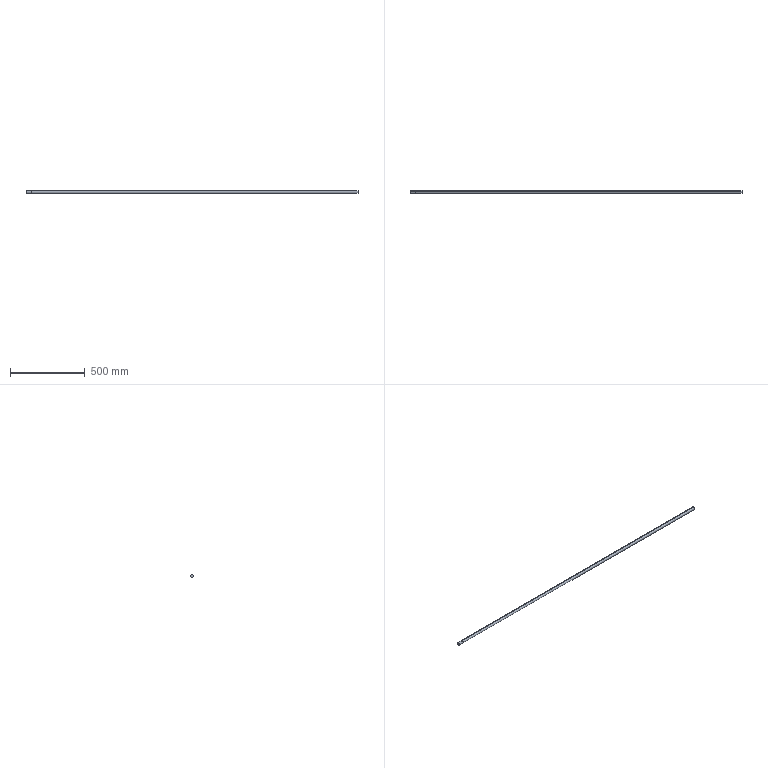Part | STEP file | _MAX100010001N_rod2 | 1 solid | 7 faces | box 2216 x 20 x 20 mm | volume 695277 mm3 | cylinder 4 | plane 3 | commonest cylinder face diameters 19 x2 20 x2
STEP:
#1=CARTESIAN_POINT('',(1723.,0.,-10.));
#2=VERTEX_POINT('',#1);
#3=CARTESIAN_POINT('',(1723.,0.,10.));
#4=VERTEX_POINT('',#3);
#5=CARTESIAN_POINT('',(1723.,0.,0.));
#6=DIRECTION('',(1.,0.,0.));
#7=DIRECTION('',(0.,0.,-1.));
#8=AXIS2_PLACEMENT_3D('',#5,#6,#7);
#9=CIRCLE('',#8,10.);
#10=EDGE_CURVE('',#2,#4,#9,.T.);
#11=ORIENTED_EDGE('',*,*,#10,.F.);
#12=CARTESIAN_POINT('',(-459.,0.,-10.));
#13=VERTEX_POINT('',#12);
#14=CARTESIAN_POINT('',(493.5,0.,-10.));
#15=DIRECTION('',(-1.,0.,0.));
#16=VECTOR('',#15,1000.);
#17=LINE('',#14,#16);
#18=EDGE_CURVE('',#2,#13,#17,.T.);
#19=ORIENTED_EDGE('',*,*,#18,.T.);
#20=CARTESIAN_POINT('',(-459.,0.,10.));
#21=VERTEX_POINT('',#20);
#22=CARTESIAN_POINT('',(-459.,0.,0.));
#23=DIRECTION('',(1.,0.,0.));
#24=DIRECTION('',(0.,0.,1.));
#25=AXIS2_PLACEMENT_3D('',#22,#23,#24);
#26=CIRCLE('',#25,10.);
#27=EDGE_CURVE('',#13,#21,#26,.T.);
#28=ORIENTED_EDGE('',*,*,#27,.T.);
#29=CARTESIAN_POINT('',(493.5,0.,10.));
#30=DIRECTION('',(-1.,0.,0.));
#31=VECTOR('',#30,1000.);
#32=LINE('',#29,#31);
#33=EDGE_CURVE('',#4,#21,#32,.T.);
#34=ORIENTED_EDGE('',*,*,#33,.F.);
#35=EDGE_LOOP('',(#11,#19,#28,#34));
#36=FACE_OUTER_BOUND('',#35,.T.);
#37=CARTESIAN_POINT('',(493.5,0.,0.));
#38=DIRECTION('',(-1.,0.,0.));
#39=DIRECTION('',(0.,0.,1.));
#40=AXIS2_PLACEMENT_3D('',#37,#38,#39);
#41=CYLINDRICAL_SURFACE('',#40,10.);
#42=ADVANCED_FACE('',(#36),#41,.T.);
#43=CARTESIAN_POINT('',(-459.,0.,9.5));
#44=VERTEX_POINT('',#43);
#45=CARTESIAN_POINT('',(-459.,0.,-9.5));
#46=VERTEX_POINT('',#45);
#47=CARTESIAN_POINT('',(-459.,0.,0.));
#48=DIRECTION('',(-1.,0.,0.));
#49=DIRECTION('',(0.,0.,1.));
#50=AXIS2_PLACEMENT_3D('',#47,#48,#49);
#51=CIRCLE('',#50,9.5);
#52=EDGE_CURVE('',#44,#46,#51,.T.);
#53=ORIENTED_EDGE('',*,*,#52,.T.);
#54=CARTESIAN_POINT('',(-493.5,0.,-9.5));
#55=VERTEX_POINT('',#54);
#56=CARTESIAN_POINT('',(493.5,0.,-9.5));
#57=DIRECTION('',(-1.,0.,0.));
#58=VECTOR('',#57,1000.);
#59=LINE('',#56,#58);
#60=EDGE_CURVE('',#46,#55,#59,.T.);
#61=ORIENTED_EDGE('',*,*,#60,.T.);
#62=CARTESIAN_POINT('',(-493.5,0.,9.5));
#63=VERTEX_POINT('',#62);
#64=CARTESIAN_POINT('',(-493.5,0.,0.));
#65=DIRECTION('',(1.,0.,0.));
#66=DIRECTION('',(0.,0.,1.));
#67=AXIS2_PLACEMENT_3D('',#64,#65,#66);
#68=CIRCLE('',#67,9.5);
#69=EDGE_CURVE('',#55,#63,#68,.T.);
#70=ORIENTED_EDGE('',*,*,#69,.T.);
#71=CARTESIAN_POINT('',(493.5,0.,9.5));
#72=DIRECTION('',(-1.,0.,0.));
#73=VECTOR('',#72,1000.);
#74=LINE('',#71,#73);
#75=EDGE_CURVE('',#44,#63,#74,.T.);
#76=ORIENTED_EDGE('',*,*,#75,.F.);
#77=EDGE_LOOP('',(#53,#61,#70,#76));
#78=FACE_OUTER_BOUND('',#77,.T.);
#79=CARTESIAN_POINT('',(493.5,0.,0.));
#80=DIRECTION('',(-1.,0.,0.));
#81=DIRECTION('',(0.,0.,1.));
#82=AXIS2_PLACEMENT_3D('',#79,#80,#81);
#83=CYLINDRICAL_SURFACE('',#82,9.5);
#84=ADVANCED_FACE('',(#78),#83,.T.);
#85=ORIENTED_EDGE('',*,*,#18,.F.);
#86=CARTESIAN_POINT('',(1723.,0.,0.));
#87=DIRECTION('',(1.,0.,0.));
#88=DIRECTION('',(0.,0.,-1.));
#89=AXIS2_PLACEMENT_3D('',#86,#87,#88);
#90=CIRCLE('',#89,10.);
#91=EDGE_CURVE('',#4,#2,#90,.T.);
#92=ORIENTED_EDGE('',*,*,#91,.F.);
#93=ORIENTED_EDGE('',*,*,#33,.T.);
#94=CARTESIAN_POINT('',(-459.,0.,0.));
#95=DIRECTION('',(1.,0.,0.));
#96=DIRECTION('',(0.,0.,1.));
#97=AXIS2_PLACEMENT_3D('',#94,#95,#96);
#98=CIRCLE('',#97,10.);
#99=EDGE_CURVE('',#21,#13,#98,.T.);
#100=ORIENTED_EDGE('',*,*,#99,.T.);
#101=EDGE_LOOP('',(#85,#92,#93,#100));
#102=FACE_OUTER_BOUND('',#101,.T.);
#103=CARTESIAN_POINT('',(493.5,0.,0.));
#104=DIRECTION('',(-1.,0.,0.));
#105=DIRECTION('',(0.,0.,1.));
#106=AXIS2_PLACEMENT_3D('',#103,#104,#105);
#107=CYLINDRICAL_SURFACE('',#106,10.);
#108=ADVANCED_FACE('',(#102),#107,.T.);
#109=ORIENTED_EDGE('',*,*,#52,.F.);
#110=CARTESIAN_POINT('',(-459.,0.,0.));
#111=DIRECTION('',(-1.,0.,0.));
#112=DIRECTION('',(0.,0.,1.));
#113=AXIS2_PLACEMENT_3D('',#110,#111,#112);
#114=CIRCLE('',#113,9.5);
#115=EDGE_CURVE('',#46,#44,#114,.T.);
#116=ORIENTED_EDGE('',*,*,#115,.F.);
#117=EDGE_LOOP('',(#109,#116));
#118=FACE_BOUND('',#117,.T.);
#119=ORIENTED_EDGE('',*,*,#99,.F.);
#120=ORIENTED_EDGE('',*,*,#27,.F.);
#121=EDGE_LOOP('',(#119,#120));
#122=FACE_OUTER_BOUND('',#121,.T.);
#123=CARTESIAN_POINT('',(-459.,9.5,0.));
#124=DIRECTION('',(1.,0.,0.));
#125=DIRECTION('',(0.,0.,-1.));
#126=AXIS2_PLACEMENT_3D('',#123,#124,#125);
#127=PLANE('',#126);
#128=ADVANCED_FACE('',(#118,#122),#127,.F.);
#129=ORIENTED_EDGE('',*,*,#60,.F.);
#130=ORIENTED_EDGE('',*,*,#115,.T.);
#131=ORIENTED_EDGE('',*,*,#75,.T.);
#132=CARTESIAN_POINT('',(-493.5,0.,0.));
#133=DIRECTION('',(1.,0.,0.));
#134=DIRECTION('',(0.,0.,1.));
#135=AXIS2_PLACEMENT_3D('',#132,#133,#134);
#136=CIRCLE('',#135,9.5);
#137=EDGE_CURVE('',#63,#55,#136,.T.);
#138=ORIENTED_EDGE('',*,*,#137,.T.);
#139=EDGE_LOOP('',(#129,#130,#131,#138));
#140=FACE_OUTER_BOUND('',#139,.T.);
#141=CARTESIAN_POINT('',(493.5,0.,0.));
#142=DIRECTION('',(-1.,0.,0.));
#143=DIRECTION('',(0.,0.,1.));
#144=AXIS2_PLACEMENT_3D('',#141,#142,#143);
#145=CYLINDRICAL_SURFACE('',#144,9.5);
#146=ADVANCED_FACE('',(#140),#145,.T.);
#147=ORIENTED_EDGE('',*,*,#137,.F.);
#148=ORIENTED_EDGE('',*,*,#69,.F.);
#149=EDGE_LOOP('',(#147,#148));
#150=FACE_OUTER_BOUND('',#149,.T.);
#151=CARTESIAN_POINT('',(-493.5,0.,0.));
#152=DIRECTION('',(1.,0.,0.));
#153=DIRECTION('',(0.,0.,-1.));
#154=AXIS2_PLACEMENT_3D('',#151,#152,#153);
#155=PLANE('',#154);
#156=ADVANCED_FACE('',(#150),#155,.F.);
#157=ORIENTED_EDGE('',*,*,#91,.T.);
#158=ORIENTED_EDGE('',*,*,#10,.T.);
#159=EDGE_LOOP('',(#157,#158));
#160=FACE_OUTER_BOUND('',#159,.T.);
#161=CARTESIAN_POINT('',(1723.,9.5,0.));
#162=DIRECTION('',(1.,0.,0.));
#163=DIRECTION('',(0.,0.,-1.));
#164=AXIS2_PLACEMENT_3D('',#161,#162,#163);
#165=PLANE('',#164);
#166=ADVANCED_FACE('',(#160),#165,.T.);
#167=CLOSED_SHELL('',(#42,#84,#108,#128,#146,#156,#166));
#168=MANIFOLD_SOLID_BREP('',#167);
#169=CARTESIAN_POINT('',(0.,0.,0.));
#170=DIRECTION('',(0.,0.,1.));
#171=DIRECTION('',(1.,0.,0.));
#172=AXIS2_PLACEMENT_3D('',#169,#170,#171);
#173=(LENGTH_UNIT()NAMED_UNIT(*)SI_UNIT(.MILLI.,.METRE.));
#174=UNCERTAINTY_MEASURE_WITH_UNIT(LENGTH_MEASURE(0.00001),#173,'','');
#175=(NAMED_UNIT(*)PLANE_ANGLE_UNIT()SI_UNIT($,.RADIAN.));
#176=(NAMED_UNIT(*)SI_UNIT($,.STERADIAN.)SOLID_ANGLE_UNIT());
#177=(GEOMETRIC_REPRESENTATION_CONTEXT(3)GLOBAL_UNCERTAINTY_ASSIGNED_CONTEXT((#174))GLOBAL_UNIT_ASSIGNED_CONTEXT((#173,#175,#176))REPRESENTATION_CONTEXT('',''));
#178=ADVANCED_BREP_SHAPE_REPRESENTATION('',(#168,#172),#177);